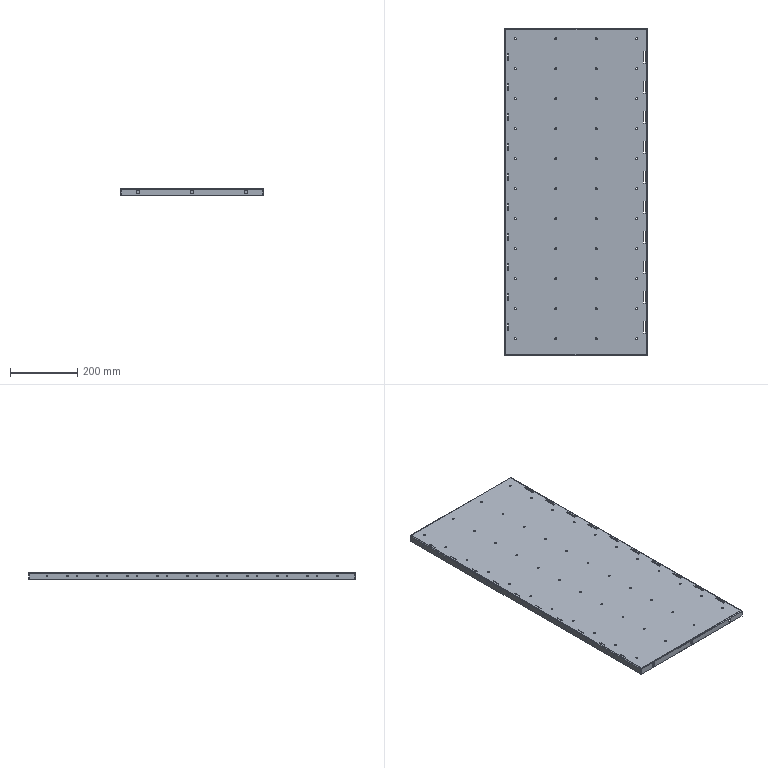Part | SolidWorks | features MirrorStock 1 | 1 solid | 300 faces | box 423 x 970 x 20 mm | volume 908267 mm3 | cylinder 182 | plane 110 | spline 8 | commonest cylinder face diameters 5.4 x168 10.5 x6 1 x4 5 x4